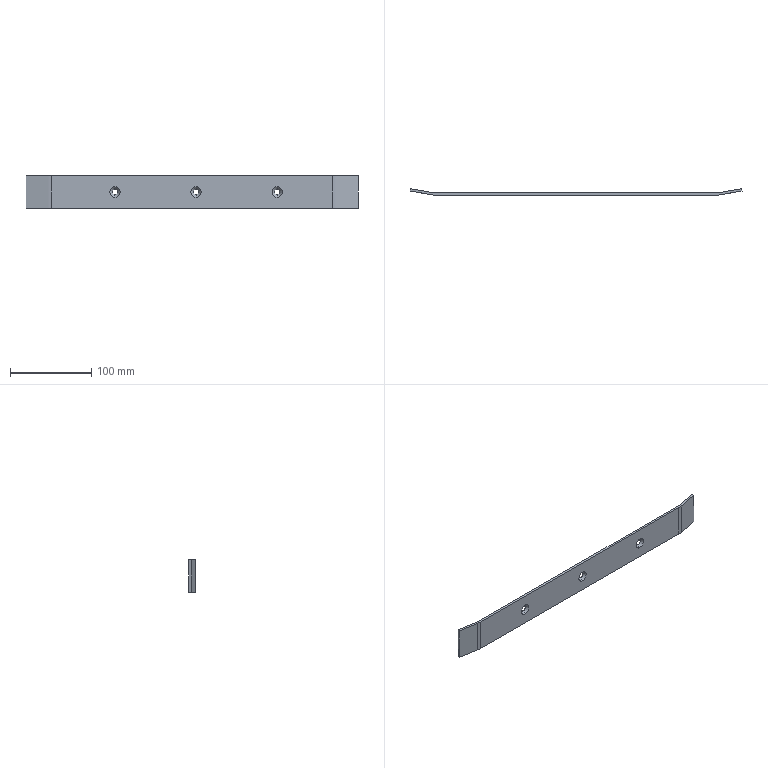Part | STEP file | 1 solid | 20 faces | box 409.088 x 8.069 x 40 mm | volume 48290 mm3 | plane 10 | cone 6 | cylinder 4 | commonest cylinder face diameters 38 x2 50 x2